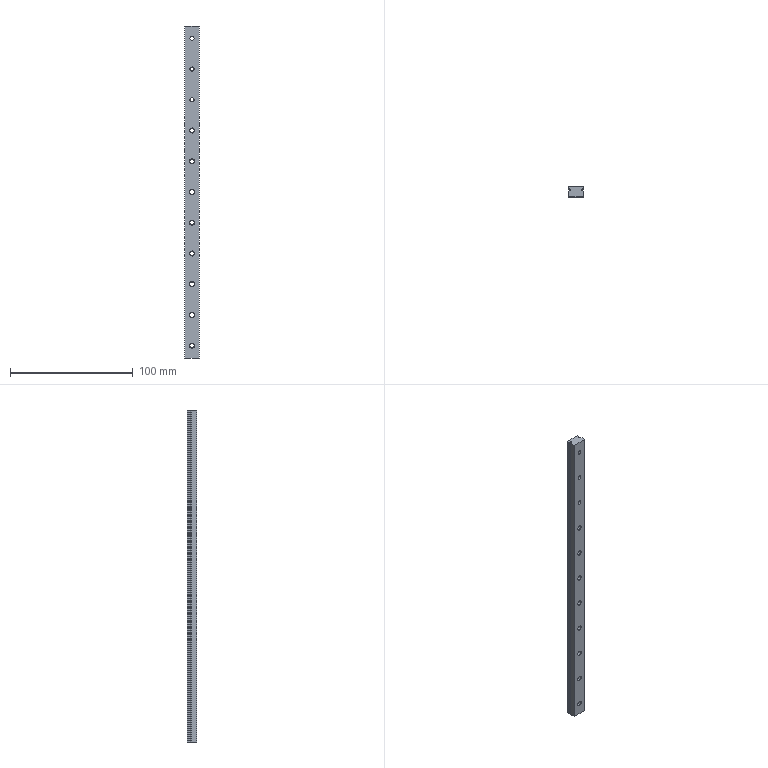Part | STEP file | C-MLG12-270 | 1 solid | 110 faces | box 12 x 8 x 270 mm | volume 22993 mm3 | cylinder 51 | cone 32 | plane 27 | commonest cylinder face diameters 6 x22 3.5 x16 3.4 x6 2.38 x4 1 x3